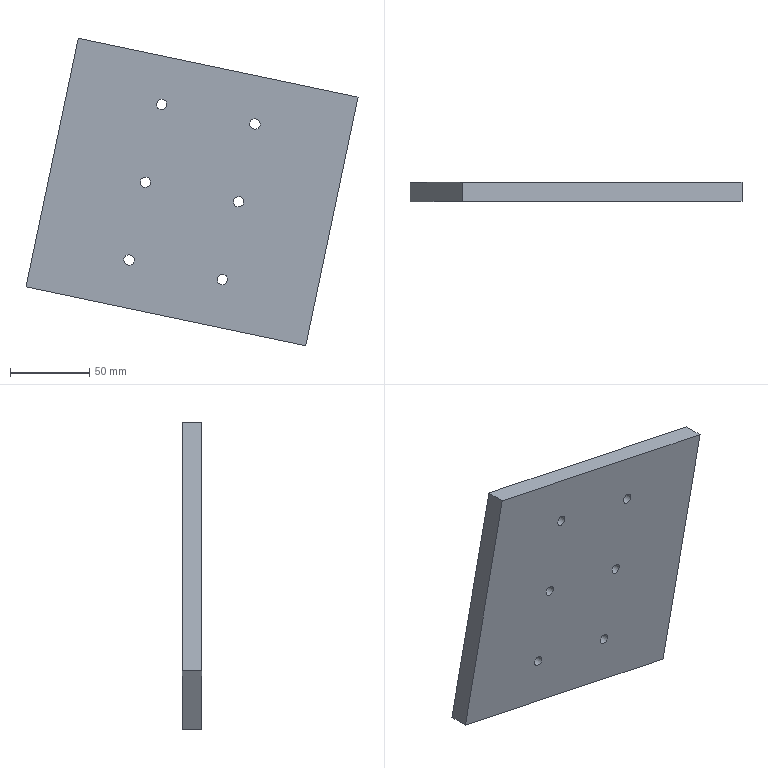Part | STEP file | SOLID | 1 solid | 24 faces | box 209.056 x 12 x 193.596 mm | volume 339030 mm3 | plane 12 | cylinder 12 | commonest cylinder face diameters 6.5 x6 13 x6
STEP:
#1=CARTESIAN_POINT('',(0.,0.,0.));
#2=DIRECTION('',(0.,0.,1.));
#3=DIRECTION('',(1.,0.,0.));
#4=AXIS2_PLACEMENT_3D('',#1,#2,#3);
#5=CARTESIAN_POINT('',(-554.568,-704.15,575.987));
#6=VERTEX_POINT('',#5);
#7=CARTESIAN_POINT('',(-560.929,-704.15,577.323));
#8=DIRECTION('',(0.,1.,0.));
#9=DIRECTION('',(0.9786,0.,-0.2056));
#10=AXIS2_PLACEMENT_3D('',#7,#8,#9);
#11=CIRCLE('',#10,6.5);
#12=CARTESIAN_POINT('',(-560.929,-704.15,577.323));
#13=DIRECTION('',(0.,1.,0.));
#14=DIRECTION('',(0.9786,0.,-0.2056));
#15=AXIS2_PLACEMENT_3D('',#12,#13,#14);
#16=PLANE('',#15);
#17=CARTESIAN_POINT('',(0.,0.));
#18=DIRECTION('',(1.,0.));
#19=AXIS2_PLACEMENT_2D('',#17,#18);
#20=CIRCLE('',#19,6.5);
#21=(GEOMETRIC_REPRESENTATION_CONTEXT(2)PARAMETRIC_REPRESENTATION_CONTEXT()REPRESENTATION_CONTEXT('',''));
#22=DEFINITIONAL_REPRESENTATION('',(#20),#21);
#23=PCURVE('',#16,#22);
#24=CARTESIAN_POINT('',(-560.929,-700.65,577.323));
#25=DIRECTION('',(0.,1.,0.));
#26=DIRECTION('',(0.9786,0.,-0.2056));
#27=AXIS2_PLACEMENT_3D('',#24,#25,#26);
#28=CYLINDRICAL_SURFACE('',#27,6.5);
#29=CARTESIAN_POINT('',(0.,-3.5));
#30=DIRECTION('',(1.,0.));
#31=VECTOR('',#30,1.);
#32=LINE('',#29,#31);
#33=(GEOMETRIC_REPRESENTATION_CONTEXT(2)PARAMETRIC_REPRESENTATION_CONTEXT()REPRESENTATION_CONTEXT('',''));
#34=DEFINITIONAL_REPRESENTATION('',(#32),#33);
#35=PCURVE('',#28,#34);
#36=SURFACE_CURVE('',#11,(#23,#35),.PCURVE_S1.);
#37=EDGE_CURVE('',#6,#6,#36,.T.);
#38=ORIENTED_EDGE('',*,*,#37,.T.);
#39=EDGE_LOOP('',(#38));
#40=FACE_BOUND('',#39,.T.);
#41=CARTESIAN_POINT('',(-564.11,-704.15,577.992));
#42=VERTEX_POINT('',#41);
#43=CARTESIAN_POINT('',(-560.929,-704.15,577.323));
#44=DIRECTION('',(0.,1.,0.));
#45=DIRECTION('',(0.9786,0.,-0.2056));
#46=AXIS2_PLACEMENT_3D('',#43,#44,#45);
#47=CIRCLE('',#46,3.25);
#48=CARTESIAN_POINT('',(0.,0.));
#49=DIRECTION('',(1.,0.));
#50=AXIS2_PLACEMENT_2D('',#48,#49);
#51=CIRCLE('',#50,3.25);
#52=(GEOMETRIC_REPRESENTATION_CONTEXT(2)PARAMETRIC_REPRESENTATION_CONTEXT()REPRESENTATION_CONTEXT('',''));
#53=DEFINITIONAL_REPRESENTATION('',(#51),#52);
#54=PCURVE('',#16,#53);
#55=CARTESIAN_POINT('',(-560.929,-982.33,577.323));
#56=DIRECTION('',(0.,1.,0.));
#57=DIRECTION('',(0.9786,0.,-0.2056));
#58=AXIS2_PLACEMENT_3D('',#55,#56,#57);
#59=CYLINDRICAL_SURFACE('',#58,3.25);
#60=CARTESIAN_POINT('',(0.,278.18));
#61=DIRECTION('',(1.,0.));
#62=VECTOR('',#61,1.);
#63=LINE('',#60,#62);
#64=(GEOMETRIC_REPRESENTATION_CONTEXT(2)PARAMETRIC_REPRESENTATION_CONTEXT()REPRESENTATION_CONTEXT('',''));
#65=DEFINITIONAL_REPRESENTATION('',(#63),#64);
#66=PCURVE('',#59,#65);
#67=SURFACE_CURVE('',#47,(#54,#66),.PCURVE_S1.);
#68=EDGE_CURVE('',#42,#42,#67,.T.);
#69=ORIENTED_EDGE('',*,*,#68,.F.);
#70=EDGE_LOOP('',(#69));
#71=FACE_BOUND('',#70,.T.);
#72=ADVANCED_FACE('',(#40,#71),#16,.T.);
#73=CARTESIAN_POINT('',(-554.568,-697.15,575.987));
#74=VERTEX_POINT('',#73);
#75=CARTESIAN_POINT('',(-560.929,-697.15,577.323));
#76=DIRECTION('',(0.,-1.,0.));
#77=DIRECTION('',(0.9786,0.,-0.2056));
#78=AXIS2_PLACEMENT_3D('',#75,#76,#77);
#79=CIRCLE('',#78,6.5);
#80=CARTESIAN_POINT('',(6.283,3.5));
#81=DIRECTION('',(-1.,0.));
#82=VECTOR('',#81,1.);
#83=LINE('',#80,#82);
#84=(GEOMETRIC_REPRESENTATION_CONTEXT(2)PARAMETRIC_REPRESENTATION_CONTEXT()REPRESENTATION_CONTEXT('',''));
#85=DEFINITIONAL_REPRESENTATION('',(#83),#84);
#86=PCURVE('',#28,#85);
#87=CARTESIAN_POINT('',(-672.195,-697.15,631.359));
#88=DIRECTION('',(0.,-1.,0.));
#89=DIRECTION('',(0.,0.,-1.));
#90=AXIS2_PLACEMENT_3D('',#87,#88,#89);
#91=PLANE('',#90);
#92=CARTESIAN_POINT('',(54.036,111.266));
#93=DIRECTION('',(0.2056,0.9786));
#94=AXIS2_PLACEMENT_2D('',#92,#93);
#95=CIRCLE('',#94,6.5);
#96=(GEOMETRIC_REPRESENTATION_CONTEXT(2)PARAMETRIC_REPRESENTATION_CONTEXT()REPRESENTATION_CONTEXT('',''));
#97=DEFINITIONAL_REPRESENTATION('',(#95),#96);
#98=PCURVE('',#91,#97);
#99=SURFACE_CURVE('',#79,(#86,#98),.PCURVE_S1.);
#100=EDGE_CURVE('',#74,#74,#99,.T.);
#101=ORIENTED_EDGE('',*,*,#100,.T.);
#102=CARTESIAN_POINT('',(-554.568,-704.15,575.987));
#103=CARTESIAN_POINT('',(-554.568,-697.15,575.987));
#104=B_SPLINE_CURVE_WITH_KNOTS('',1,(#102,#103),.UNSPECIFIED.,.F.,.F.,(2,2),(-3.5,3.5),.PIECEWISE_BEZIER_KNOTS.);
#105=CARTESIAN_POINT('',(0.,0.));
#106=DIRECTION('',(0.,1.));
#107=VECTOR('',#106,1.);
#108=LINE('',#105,#107);
#109=(GEOMETRIC_REPRESENTATION_CONTEXT(2)PARAMETRIC_REPRESENTATION_CONTEXT()REPRESENTATION_CONTEXT('',''));
#110=DEFINITIONAL_REPRESENTATION('',(#108),#109);
#111=PCURVE('',#28,#110);
#112=CARTESIAN_POINT('',(6.283,0.));
#113=DIRECTION('',(0.,1.));
#114=VECTOR('',#113,1.);
#115=LINE('',#112,#114);
#116=(GEOMETRIC_REPRESENTATION_CONTEXT(2)PARAMETRIC_REPRESENTATION_CONTEXT()REPRESENTATION_CONTEXT('',''));
#117=DEFINITIONAL_REPRESENTATION('',(#115),#116);
#118=PCURVE('',#28,#117);
#119=SEAM_CURVE('',#104,(#111,#118),.PCURVE_S1.);
#120=EDGE_CURVE('',#6,#74,#119,.T.);
#121=ORIENTED_EDGE('',*,*,#120,.F.);
#122=ORIENTED_EDGE('',*,*,#37,.T.);
#123=ORIENTED_EDGE('',*,*,#120,.T.);
#124=EDGE_LOOP('',(#101,#121,#122,#123));
#125=FACE_BOUND('',#124,.F.);
#126=ADVANCED_FACE('',(#125),#28,.F.);
#127=CARTESIAN_POINT('',(-564.11,-709.15,577.992));
#128=VERTEX_POINT('',#127);
#129=CARTESIAN_POINT('',(-560.929,-709.15,577.323));
#130=DIRECTION('',(0.,1.,0.));
#131=DIRECTION('',(0.9786,0.,-0.2056));
#132=AXIS2_PLACEMENT_3D('',#129,#130,#131);
#133=CIRCLE('',#132,3.25);
#134=CARTESIAN_POINT('',(0.,273.18));
#135=DIRECTION('',(1.,0.));
#136=VECTOR('',#135,1.);
#137=LINE('',#134,#136);
#138=(GEOMETRIC_REPRESENTATION_CONTEXT(2)PARAMETRIC_REPRESENTATION_CONTEXT()REPRESENTATION_CONTEXT('',''));
#139=DEFINITIONAL_REPRESENTATION('',(#137),#138);
#140=PCURVE('',#59,#139);
#141=CARTESIAN_POINT('',(-554.191,-709.15,463.505));
#142=DIRECTION('',(0.,1.,0.));
#143=DIRECTION('',(0.,0.,1.));
#144=AXIS2_PLACEMENT_3D('',#141,#142,#143);
#145=PLANE('',#144);
#146=CARTESIAN_POINT('',(113.818,-6.738));
#147=DIRECTION('',(-0.2056,0.9786));
#148=AXIS2_PLACEMENT_2D('',#146,#147);
#149=CIRCLE('',#148,3.25);
#150=(GEOMETRIC_REPRESENTATION_CONTEXT(2)PARAMETRIC_REPRESENTATION_CONTEXT()REPRESENTATION_CONTEXT('',''));
#151=DEFINITIONAL_REPRESENTATION('',(#149),#150);
#152=PCURVE('',#145,#151);
#153=SURFACE_CURVE('',#133,(#140,#152),.PCURVE_S1.);
#154=EDGE_CURVE('',#128,#128,#153,.T.);
#155=ORIENTED_EDGE('',*,*,#154,.T.);
#156=CARTESIAN_POINT('',(-564.11,-709.15,577.992));
#157=CARTESIAN_POINT('',(-564.11,-704.15,577.992));
#158=B_SPLINE_CURVE_WITH_KNOTS('',1,(#156,#157),.UNSPECIFIED.,.F.,.F.,(2,2),(273.18,278.18),.PIECEWISE_BEZIER_KNOTS.);
#159=CARTESIAN_POINT('',(9.425,0.));
#160=DIRECTION('',(0.,1.));
#161=VECTOR('',#160,1.);
#162=LINE('',#159,#161);
#163=(GEOMETRIC_REPRESENTATION_CONTEXT(2)PARAMETRIC_REPRESENTATION_CONTEXT()REPRESENTATION_CONTEXT('',''));
#164=DEFINITIONAL_REPRESENTATION('',(#162),#163);
#165=PCURVE('',#59,#164);
#166=CARTESIAN_POINT('',(3.142,0.));
#167=DIRECTION('',(0.,1.));
#168=VECTOR('',#167,1.);
#169=LINE('',#166,#168);
#170=(GEOMETRIC_REPRESENTATION_CONTEXT(2)PARAMETRIC_REPRESENTATION_CONTEXT()REPRESENTATION_CONTEXT('',''));
#171=DEFINITIONAL_REPRESENTATION('',(#169),#170);
#172=PCURVE('',#59,#171);
#173=SEAM_CURVE('',#158,(#165,#172),.PCURVE_S1.);
#174=EDGE_CURVE('',#128,#42,#173,.T.);
#175=ORIENTED_EDGE('',*,*,#174,.T.);
#176=ORIENTED_EDGE('',*,*,#68,.F.);
#177=ORIENTED_EDGE('',*,*,#174,.F.);
#178=EDGE_LOOP('',(#155,#175,#176,#177));
#179=FACE_BOUND('',#178,.F.);
#180=ADVANCED_FACE('',(#179),#59,.F.);
#181=CARTESIAN_POINT('',(-564.85,-704.15,527.055));
#182=VERTEX_POINT('',#181);
#183=CARTESIAN_POINT('',(-571.211,-704.15,528.392));
#184=DIRECTION('',(0.,1.,0.));
#185=DIRECTION('',(0.9786,0.,-0.2056));
#186=AXIS2_PLACEMENT_3D('',#183,#184,#185);
#187=CIRCLE('',#186,6.5);
#188=CARTESIAN_POINT('',(-571.211,-704.15,528.392));
#189=DIRECTION('',(0.,1.,0.));
#190=DIRECTION('',(0.9786,0.,-0.2056));
#191=AXIS2_PLACEMENT_3D('',#188,#189,#190);
#192=PLANE('',#191);
#193=CARTESIAN_POINT('',(0.,0.));
#194=DIRECTION('',(1.,0.));
#195=AXIS2_PLACEMENT_2D('',#193,#194);
#196=CIRCLE('',#195,6.5);
#197=(GEOMETRIC_REPRESENTATION_CONTEXT(2)PARAMETRIC_REPRESENTATION_CONTEXT()REPRESENTATION_CONTEXT('',''));
#198=DEFINITIONAL_REPRESENTATION('',(#196),#197);
#199=PCURVE('',#192,#198);
#200=CARTESIAN_POINT('',(-571.211,-700.65,528.392));
#201=DIRECTION('',(0.,1.,0.));
#202=DIRECTION('',(0.9786,0.,-0.2056));
#203=AXIS2_PLACEMENT_3D('',#200,#201,#202);
#204=CYLINDRICAL_SURFACE('',#203,6.5);
#205=CARTESIAN_POINT('',(0.,-3.5));
#206=DIRECTION('',(1.,0.));
#207=VECTOR('',#206,1.);
#208=LINE('',#205,#207);
#209=(GEOMETRIC_REPRESENTATION_CONTEXT(2)PARAMETRIC_REPRESENTATION_CONTEXT()REPRESENTATION_CONTEXT('',''));
#210=DEFINITIONAL_REPRESENTATION('',(#208),#209);
#211=PCURVE('',#204,#210);
#212=SURFACE_CURVE('',#187,(#199,#211),.PCURVE_S1.);
#213=EDGE_CURVE('',#182,#182,#212,.T.);
#214=ORIENTED_EDGE('',*,*,#213,.T.);
#215=EDGE_LOOP('',(#214));
#216=FACE_BOUND('',#215,.T.);
#217=CARTESIAN_POINT('',(-574.392,-704.15,529.06));
#218=VERTEX_POINT('',#217);
#219=CARTESIAN_POINT('',(-571.211,-704.15,528.392));
#220=DIRECTION('',(0.,1.,0.));
#221=DIRECTION('',(0.9786,0.,-0.2056));
#222=AXIS2_PLACEMENT_3D('',#219,#220,#221);
#223=CIRCLE('',#222,3.25);
#224=CARTESIAN_POINT('',(0.,0.));
#225=DIRECTION('',(1.,0.));
#226=AXIS2_PLACEMENT_2D('',#224,#225);
#227=CIRCLE('',#226,3.25);
#228=(GEOMETRIC_REPRESENTATION_CONTEXT(2)PARAMETRIC_REPRESENTATION_CONTEXT()REPRESENTATION_CONTEXT('',''));
#229=DEFINITIONAL_REPRESENTATION('',(#227),#228);
#230=PCURVE('',#192,#229);
#231=CARTESIAN_POINT('',(-571.211,-982.33,528.392));
#232=DIRECTION('',(0.,1.,0.));
#233=DIRECTION('',(0.9786,0.,-0.2056));
#234=AXIS2_PLACEMENT_3D('',#231,#232,#233);
#235=CYLINDRICAL_SURFACE('',#234,3.25);
#236=CARTESIAN_POINT('',(0.,278.18));
#237=DIRECTION('',(1.,0.));
#238=VECTOR('',#237,1.);
#239=LINE('',#236,#238);
#240=(GEOMETRIC_REPRESENTATION_CONTEXT(2)PARAMETRIC_REPRESENTATION_CONTEXT()REPRESENTATION_CONTEXT('',''));
#241=DEFINITIONAL_REPRESENTATION('',(#239),#240);
#242=PCURVE('',#235,#241);
#243=SURFACE_CURVE('',#223,(#230,#242),.PCURVE_S1.);
#244=EDGE_CURVE('',#218,#218,#243,.T.);
#245=ORIENTED_EDGE('',*,*,#244,.F.);
#246=EDGE_LOOP('',(#245));
#247=FACE_BOUND('',#246,.T.);
#248=ADVANCED_FACE('',(#216,#247),#192,.T.);
#249=CARTESIAN_POINT('',(-564.85,-697.15,527.055));
#250=VERTEX_POINT('',#249);
#251=CARTESIAN_POINT('',(-571.211,-697.15,528.392));
#252=DIRECTION('',(0.,-1.,0.));
#253=DIRECTION('',(0.9786,0.,-0.2056));
#254=AXIS2_PLACEMENT_3D('',#251,#252,#253);
#255=CIRCLE('',#254,6.5);
#256=CARTESIAN_POINT('',(6.283,3.5));
#257=DIRECTION('',(-1.,0.));
#258=VECTOR('',#257,1.);
#259=LINE('',#256,#258);
#260=(GEOMETRIC_REPRESENTATION_CONTEXT(2)PARAMETRIC_REPRESENTATION_CONTEXT()REPRESENTATION_CONTEXT('',''));
#261=DEFINITIONAL_REPRESENTATION('',(#259),#260);
#262=PCURVE('',#204,#261);
#263=CARTESIAN_POINT('',(102.967,100.984));
#264=DIRECTION('',(0.2056,0.9786));
#265=AXIS2_PLACEMENT_2D('',#263,#264);
#266=CIRCLE('',#265,6.5);
#267=(GEOMETRIC_REPRESENTATION_CONTEXT(2)PARAMETRIC_REPRESENTATION_CONTEXT()REPRESENTATION_CONTEXT('',''));
#268=DEFINITIONAL_REPRESENTATION('',(#266),#267);
#269=PCURVE('',#91,#268);
#270=SURFACE_CURVE('',#255,(#262,#269),.PCURVE_S1.);
#271=EDGE_CURVE('',#250,#250,#270,.T.);
#272=ORIENTED_EDGE('',*,*,#271,.T.);
#273=CARTESIAN_POINT('',(-564.85,-704.15,527.055));
#274=CARTESIAN_POINT('',(-564.85,-697.15,527.055));
#275=B_SPLINE_CURVE_WITH_KNOTS('',1,(#273,#274),.UNSPECIFIED.,.F.,.F.,(2,2),(-3.5,3.5),.PIECEWISE_BEZIER_KNOTS.);
#276=CARTESIAN_POINT('',(0.,0.));
#277=DIRECTION('',(0.,1.));
#278=VECTOR('',#277,1.);
#279=LINE('',#276,#278);
#280=(GEOMETRIC_REPRESENTATION_CONTEXT(2)PARAMETRIC_REPRESENTATION_CONTEXT()REPRESENTATION_CONTEXT('',''));
#281=DEFINITIONAL_REPRESENTATION('',(#279),#280);
#282=PCURVE('',#204,#281);
#283=CARTESIAN_POINT('',(6.283,0.));
#284=DIRECTION('',(0.,1.));
#285=VECTOR('',#284,1.);
#286=LINE('',#283,#285);
#287=(GEOMETRIC_REPRESENTATION_CONTEXT(2)PARAMETRIC_REPRESENTATION_CONTEXT()REPRESENTATION_CONTEXT('',''));
#288=DEFINITIONAL_REPRESENTATION('',(#286),#287);
#289=PCURVE('',#204,#288);
#290=SEAM_CURVE('',#275,(#282,#289),.PCURVE_S1.);
#291=EDGE_CURVE('',#182,#250,#290,.T.);
#292=ORIENTED_EDGE('',*,*,#291,.F.);
#293=ORIENTED_EDGE('',*,*,#213,.T.);
#294=ORIENTED_EDGE('',*,*,#291,.T.);
#295=EDGE_LOOP('',(#272,#292,#293,#294));
#296=FACE_BOUND('',#295,.F.);
#297=ADVANCED_FACE('',(#296),#204,.F.);
#298=CARTESIAN_POINT('',(-574.392,-709.15,529.06));
#299=VERTEX_POINT('',#298);
#300=CARTESIAN_POINT('',(-571.211,-709.15,528.392));
#301=DIRECTION('',(0.,1.,0.));
#302=DIRECTION('',(0.9786,0.,-0.2056));
#303=AXIS2_PLACEMENT_3D('',#300,#301,#302);
#304=CIRCLE('',#303,3.25);
#305=CARTESIAN_POINT('',(0.,273.18));
#306=DIRECTION('',(1.,0.));
#307=VECTOR('',#306,1.);
#308=LINE('',#305,#307);
#309=(GEOMETRIC_REPRESENTATION_CONTEXT(2)PARAMETRIC_REPRESENTATION_CONTEXT()REPRESENTATION_CONTEXT('',''));
#310=DEFINITIONAL_REPRESENTATION('',(#308),#309);
#311=PCURVE('',#235,#310);
#312=CARTESIAN_POINT('',(64.887,-17.02));
#313=DIRECTION('',(-0.2056,0.9786));
#314=AXIS2_PLACEMENT_2D('',#312,#313);
#315=CIRCLE('',#314,3.25);
#316=(GEOMETRIC_REPRESENTATION_CONTEXT(2)PARAMETRIC_REPRESENTATION_CONTEXT()REPRESENTATION_CONTEXT('',''));
#317=DEFINITIONAL_REPRESENTATION('',(#315),#316);
#318=PCURVE('',#145,#317);
#319=SURFACE_CURVE('',#304,(#311,#318),.PCURVE_S1.);
#320=EDGE_CURVE('',#299,#299,#319,.T.);
#321=ORIENTED_EDGE('',*,*,#320,.T.);
#322=CARTESIAN_POINT('',(-574.392,-709.15,529.06));
#323=CARTESIAN_POINT('',(-574.392,-704.15,529.06));
#324=B_SPLINE_CURVE_WITH_KNOTS('',1,(#322,#323),.UNSPECIFIED.,.F.,.F.,(2,2),(273.18,278.18),.PIECEWISE_BEZIER_KNOTS.);
#325=CARTESIAN_POINT('',(9.425,0.));
#326=DIRECTION('',(0.,1.));
#327=VECTOR('',#326,1.);
#328=LINE('',#325,#327);
#329=(GEOMETRIC_REPRESENTATION_CONTEXT(2)PARAMETRIC_REPRESENTATION_CONTEXT()REPRESENTATION_CONTEXT('',''));
#330=DEFINITIONAL_REPRESENTATION('',(#328),#329);
#331=PCURVE('',#235,#330);
#332=CARTESIAN_POINT('',(3.142,0.));
#333=DIRECTION('',(0.,1.));
#334=VECTOR('',#333,1.);
#335=LINE('',#332,#334);
#336=(GEOMETRIC_REPRESENTATION_CONTEXT(2)PARAMETRIC_REPRESENTATION_CONTEXT()REPRESENTATION_CONTEXT('',''));
#337=DEFINITIONAL_REPRESENTATION('',(#335),#336);
#338=PCURVE('',#235,#337);
#339=SEAM_CURVE('',#324,(#331,#338),.PCURVE_S1.);
#340=EDGE_CURVE('',#299,#218,#339,.T.);
#341=ORIENTED_EDGE('',*,*,#340,.T.);
#342=ORIENTED_EDGE('',*,*,#244,.F.);
#343=ORIENTED_EDGE('',*,*,#340,.F.);
#344=EDGE_LOOP('',(#321,#341,#342,#343));
#345=FACE_BOUND('',#344,.F.);
#346=ADVANCED_FACE('',(#345),#235,.F.);
#347=CARTESIAN_POINT('',(-575.132,-704.15,478.124));
#348=VERTEX_POINT('',#347);
#349=CARTESIAN_POINT('',(-581.494,-704.15,479.46));
#350=DIRECTION('',(0.,1.,0.));
#351=DIRECTION('',(0.9786,0.,-0.2056));
#352=AXIS2_PLACEMENT_3D('',#349,#350,#351);
#353=CIRCLE('',#352,6.5);
#354=CARTESIAN_POINT('',(-581.494,-704.15,479.46));
#355=DIRECTION('',(0.,1.,0.));
#356=DIRECTION('',(0.9786,0.,-0.2056));
#357=AXIS2_PLACEMENT_3D('',#354,#355,#356);
#358=PLANE('',#357);
#359=CARTESIAN_POINT('',(0.,0.));
#360=DIRECTION('',(1.,0.));
#361=AXIS2_PLACEMENT_2D('',#359,#360);
#362=CIRCLE('',#361,6.5);
#363=(GEOMETRIC_REPRESENTATION_CONTEXT(2)PARAMETRIC_REPRESENTATION_CONTEXT()REPRESENTATION_CONTEXT('',''));
#364=DEFINITIONAL_REPRESENTATION('',(#362),#363);
#365=PCURVE('',#358,#364);
#366=CARTESIAN_POINT('',(-581.494,-700.65,479.46));
#367=DIRECTION('',(0.,1.,0.));
#368=DIRECTION('',(0.9786,0.,-0.2056));
#369=AXIS2_PLACEMENT_3D('',#366,#367,#368);
#370=CYLINDRICAL_SURFACE('',#369,6.5);
#371=CARTESIAN_POINT('',(0.,-3.5));
#372=DIRECTION('',(1.,0.));
#373=VECTOR('',#372,1.);
#374=LINE('',#371,#373);
#375=(GEOMETRIC_REPRESENTATION_CONTEXT(2)PARAMETRIC_REPRESENTATION_CONTEXT()REPRESENTATION_CONTEXT('',''));
#376=DEFINITIONAL_REPRESENTATION('',(#374),#375);
#377=PCURVE('',#370,#376);
#378=SURFACE_CURVE('',#353,(#365,#377),.PCURVE_S1.);
#379=EDGE_CURVE('',#348,#348,#378,.T.);
#380=ORIENTED_EDGE('',*,*,#379,.T.);
#381=EDGE_LOOP('',(#380));
#382=FACE_BOUND('',#381,.T.);
#383=CARTESIAN_POINT('',(-584.674,-704.15,480.129));
#384=VERTEX_POINT('',#383);
#385=CARTESIAN_POINT('',(-581.494,-704.15,479.46));
#386=DIRECTION('',(0.,1.,0.));
#387=DIRECTION('',(0.9786,0.,-0.2056));
#388=AXIS2_PLACEMENT_3D('',#385,#386,#387);
#389=CIRCLE('',#388,3.25);
#390=CARTESIAN_POINT('',(0.,0.));
#391=DIRECTION('',(1.,0.));
#392=AXIS2_PLACEMENT_2D('',#390,#391);
#393=CIRCLE('',#392,3.25);
#394=(GEOMETRIC_REPRESENTATION_CONTEXT(2)PARAMETRIC_REPRESENTATION_CONTEXT()REPRESENTATION_CONTEXT('',''));
#395=DEFINITIONAL_REPRESENTATION('',(#393),#394);
#396=PCURVE('',#358,#395);
#397=CARTESIAN_POINT('',(-581.494,-982.33,479.46));
#398=DIRECTION('',(0.,1.,0.));
#399=DIRECTION('',(0.9786,0.,-0.2056));
#400=AXIS2_PLACEMENT_3D('',#397,#398,#399);
#401=CYLINDRICAL_SURFACE('',#400,3.25);
#402=CARTESIAN_POINT('',(0.,278.18));
#403=DIRECTION('',(1.,0.));
#404=VECTOR('',#403,1.);
#405=LINE('',#402,#404);
#406=(GEOMETRIC_REPRESENTATION_CONTEXT(2)PARAMETRIC_REPRESENTATION_CONTEXT()REPRESENTATION_CONTEXT('',''));
#407=DEFINITIONAL_REPRESENTATION('',(#405),#406);
#408=PCURVE('',#401,#407);
#409=SURFACE_CURVE('',#389,(#396,#408),.PCURVE_S1.);
#410=EDGE_CURVE('',#384,#384,#409,.T.);
#411=ORIENTED_EDGE('',*,*,#410,.F.);
#412=EDGE_LOOP('',(#411));
#413=FACE_BOUND('',#412,.T.);
#414=ADVANCED_FACE('',(#382,#413),#358,.T.);
#415=CARTESIAN_POINT('',(-575.132,-697.15,478.124));
#416=VERTEX_POINT('',#415);
#417=CARTESIAN_POINT('',(-581.494,-697.15,479.46));
#418=DIRECTION('',(0.,-1.,0.));
#419=DIRECTION('',(0.9786,0.,-0.2056));
#420=AXIS2_PLACEMENT_3D('',#417,#418,#419);
#421=CIRCLE('',#420,6.5);
#422=CARTESIAN_POINT('',(6.283,3.5));
#423=DIRECTION('',(-1.,0.));
#424=VECTOR('',#423,1.);
#425=LINE('',#422,#424);
#426=(GEOMETRIC_REPRESENTATION_CONTEXT(2)PARAMETRIC_REPRESENTATION_CONTEXT()REPRESENTATION_CONTEXT('',''));
#427=DEFINITIONAL_REPRESENTATION('',(#425),#426);
#428=PCURVE('',#370,#427);
#429=CARTESIAN_POINT('',(151.899,90.702));
#430=DIRECTION('',(0.2056,0.9786));
#431=AXIS2_PLACEMENT_2D('',#429,#430);
#432=CIRCLE('',#431,6.5);
#433=(GEOMETRIC_REPRESENTATION_CONTEXT(2)PARAMETRIC_REPRESENTATION_CONTEXT()REPRESENTATION_CONTEXT('',''));
#434=DEFINITIONAL_REPRESENTATION('',(#432),#433);
#435=PCURVE('',#91,#434);
#436=SURFACE_CURVE('',#421,(#428,#435),.PCURVE_S1.);
#437=EDGE_CURVE('',#416,#416,#436,.T.);
#438=ORIENTED_EDGE('',*,*,#437,.T.);
#439=CARTESIAN_POINT('',(-575.132,-704.15,478.124));
#440=CARTESIAN_POINT('',(-575.132,-697.15,478.124));
#441=B_SPLINE_CURVE_WITH_KNOTS('',1,(#439,#440),.UNSPECIFIED.,.F.,.F.,(2,2),(-3.5,3.5),.PIECEWISE_BEZIER_KNOTS.);
#442=CARTESIAN_POINT('',(0.,0.));
#443=DIRECTION('',(0.,1.));
#444=VECTOR('',#443,1.);
#445=LINE('',#442,#444);
#446=(GEOMETRIC_REPRESENTATION_CONTEXT(2)PARAMETRIC_REPRESENTATION_CONTEXT()REPRESENTATION_CONTEXT('',''));
#447=DEFINITIONAL_REPRESENTATION('',(#445),#446);
#448=PCURVE('',#370,#447);
#449=CARTESIAN_POINT('',(6.283,0.));
#450=DIRECTION('',(0.,1.));
#451=VECTOR('',#450,1.);
#452=LINE('',#449,#451);
#453=(GEOMETRIC_REPRESENTATION_CONTEXT(2)PARAMETRIC_REPRESENTATION_CONTEXT()REPRESENTATION_CONTEXT('',''));
#454=DEFINITIONAL_REPRESENTATION('',(#452),#453);
#455=PCURVE('',#370,#454);
#456=SEAM_CURVE('',#441,(#448,#455),.PCURVE_S1.);
#457=EDGE_CURVE('',#348,#416,#456,.T.);
#458=ORIENTED_EDGE('',*,*,#457,.F.);
#459=ORIENTED_EDGE('',*,*,#379,.T.);
#460=ORIENTED_EDGE('',*,*,#457,.T.);
#461=EDGE_LOOP('',(#438,#458,#459,#460));
#462=FACE_BOUND('',#461,.F.);
#463=ADVANCED_FACE('',(#462),#370,.F.);
#464=CARTESIAN_POINT('',(-584.674,-709.15,480.129));
#465=VERTEX_POINT('',#464);
#466=CARTESIAN_POINT('',(-581.494,-709.15,479.46));
#467=DIRECTION('',(0.,1.,0.));
#468=DIRECTION('',(0.9786,0.,-0.2056));
#469=AXIS2_PLACEMENT_3D('',#466,#467,#468);
#470=CIRCLE('',#469,3.25);
#471=CARTESIAN_POINT('',(0.,273.18));
#472=DIRECTION('',(1.,0.));
#473=VECTOR('',#472,1.);
#474=LINE('',#471,#473);
#475=(GEOMETRIC_REPRESENTATION_CONTEXT(2)PARAMETRIC_REPRESENTATION_CONTEXT()REPRESENTATION_CONTEXT('',''));
#476=DEFINITIONAL_REPRESENTATION('',(#474),#475);
#477=PCURVE('',#401,#476);
#478=CARTESIAN_POINT('',(15.956,-27.302));
#479=DIRECTION('',(-0.2056,0.9786));
#480=AXIS2_PLACEMENT_2D('',#478,#479);
#481=CIRCLE('',#480,3.25);
#482=(GEOMETRIC_REPRESENTATION_CONTEXT(2)PARAMETRIC_REPRESENTATION_CONTEXT()REPRESENTATION_CONTEXT('',''));
#483=DEFINITIONAL_REPRESENTATION('',(#481),#482);
#484=PCURVE('',#145,#483);
#485=SURFACE_CURVE('',#470,(#477,#484),.PCURVE_S1.);
#486=EDGE_CURVE('',#465,#465,#485,.T.);
#487=ORIENTED_EDGE('',*,*,#486,.T.);
#488=CARTESIAN_POINT('',(-584.674,-709.15,480.129));
#489=CARTESIAN_POINT('',(-584.674,-704.15,480.129));
#490=B_SPLINE_CURVE_WITH_KNOTS('',1,(#488,#489),.UNSPECIFIED.,.F.,.F.,(2,2),(273.18,278.18),.PIECEWISE_BEZIER_KNOTS.);
#491=CARTESIAN_POINT('',(9.425,0.));
#492=DIRECTION('',(0.,1.));
#493=VECTOR('',#492,1.);
#494=LINE('',#491,#493);
#495=(GEOMETRIC_REPRESENTATION_CONTEXT(2)PARAMETRIC_REPRESENTATION_CONTEXT()REPRESENTATION_CONTEXT('',''));
#496=DEFINITIONAL_REPRESENTATION('',(#494),#495);
#497=PCURVE('',#401,#496);
#498=CARTESIAN_POINT('',(3.142,0.));
#499=DIRECTION('',(0.,1.));
#500=VECTOR('',#499,1.);
#501=LINE('',#498,#500);
#502=(GEOMETRIC_REPRESENTATION_CONTEXT(2)PARAMETRIC_REPRESENTATION_CONTEXT()REPRESENTATION_CONTEXT('',''));
#503=DEFINITIONAL_REPRESENTATION('',(#501),#502);
#504=PCURVE('',#401,#503);
#505=SEAM_CURVE('',#490,(#497,#504),.PCURVE_S1.);
#506=EDGE_CURVE('',#465,#384,#505,.T.);
#507=ORIENTED_EDGE('',*,*,#506,.T.);
#508=ORIENTED_EDGE('',*,*,#410,.F.);
#509=ORIENTED_EDGE('',*,*,#506,.F.);
#510=EDGE_LOOP('',(#487,#507,#508,#509));
#511=FACE_BOUND('',#510,.F.);
#512=ADVANCED_FACE('',(#511),#401,.F.);
#513=CARTESIAN_POINT('',(-633.85,-704.15,490.462));
#514=VERTEX_POINT('',#513);
#515=CARTESIAN_POINT('',(-640.211,-704.15,491.799));
#516=DIRECTION('',(0.,1.,0.));
#517=DIRECTION('',(0.9786,0.,-0.2056));
#518=AXIS2_PLACEMENT_3D('',#515,#516,#517);
#519=CIRCLE('',#518,6.5);
#520=CARTESIAN_POINT('',(-640.211,-704.15,491.799));
#521=DIRECTION('',(0.,1.,0.));
#522=DIRECTION('',(0.9786,0.,-0.2056));
#523=AXIS2_PLACEMENT_3D('',#520,#521,#522);
#524=PLANE('',#523);
#525=CARTESIAN_POINT('',(0.,0.));
#526=DIRECTION('',(1.,0.));
#527=AXIS2_PLACEMENT_2D('',#525,#526);
#528=CIRCLE('',#527,6.5);
#529=(GEOMETRIC_REPRESENTATION_CONTEXT(2)PARAMETRIC_REPRESENTATION_CONTEXT()REPRESENTATION_CONTEXT('',''));
#530=DEFINITIONAL_REPRESENTATION('',(#528),#529);
#531=PCURVE('',#524,#530);
#532=CARTESIAN_POINT('',(-640.211,-700.65,491.799));
#533=DIRECTION('',(0.,1.,0.));
#534=DIRECTION('',(0.9786,0.,-0.2056));
#535=AXIS2_PLACEMENT_3D('',#532,#533,#534);
#536=CYLINDRICAL_SURFACE('',#535,6.5);
#537=CARTESIAN_POINT('',(0.,-3.5));
#538=DIRECTION('',(1.,0.));
#539=VECTOR('',#538,1.);
#540=LINE('',#537,#539);
#541=(GEOMETRIC_REPRESENTATION_CONTEXT(2)PARAMETRIC_REPRESENTATION_CONTEXT()REPRESENTATION_CONTEXT('',''));
#542=DEFINITIONAL_REPRESENTATION('',(#540),#541);
#543=PCURVE('',#536,#542);
#544=SURFACE_CURVE('',#519,(#531,#543),.PCURVE_S1.);
#545=EDGE_CURVE('',#514,#514,#544,.T.);
#546=ORIENTED_EDGE('',*,*,#545,.T.);
#547=EDGE_LOOP('',(#546));
#548=FACE_BOUND('',#547,.T.);
#549=CARTESIAN_POINT('',(-643.392,-704.15,492.467));
#550=VERTEX_POINT('',#549);
#551=CARTESIAN_POINT('',(-640.211,-704.15,491.799));
#552=DIRECTION('',(0.,1.,0.));
#553=DIRECTION('',(0.9786,0.,-0.2056));
#554=AXIS2_PLACEMENT_3D('',#551,#552,#553);
#555=CIRCLE('',#554,3.25);
#556=CARTESIAN_POINT('',(0.,0.));
#557=DIRECTION('',(1.,0.));
#558=AXIS2_PLACEMENT_2D('',#556,#557);
#559=CIRCLE('',#558,3.25);
#560=(GEOMETRIC_REPRESENTATION_CONTEXT(2)PARAMETRIC_REPRESENTATION_CONTEXT()REPRESENTATION_CONTEXT('',''));
#561=DEFINITIONAL_REPRESENTATION('',(#559),#560);
#562=PCURVE('',#524,#561);
#563=CARTESIAN_POINT('',(-640.211,-982.33,491.799));
#564=DIRECTION('',(0.,1.,0.));
#565=DIRECTION('',(0.9786,0.,-0.2056));
#566=AXIS2_PLACEMENT_3D('',#563,#564,#565);
#567=CYLINDRICAL_SURFACE('',#566,3.25);
#568=CARTESIAN_POINT('',(0.,278.18));
#569=DIRECTION('',(1.,0.));
#570=VECTOR('',#569,1.);
#571=LINE('',#568,#570);
#572=(GEOMETRIC_REPRESENTATION_CONTEXT(2)PARAMETRIC_REPRESENTATION_CONTEXT()REPRESENTATION_CONTEXT('',''));
#573=DEFINITIONAL_REPRESENTATION('',(#571),#572);
#574=PCURVE('',#567,#573);
#575=SURFACE_CURVE('',#555,(#562,#574),.PCURVE_S1.);
#576=EDGE_CURVE('',#550,#550,#575,.T.);
#577=ORIENTED_EDGE('',*,*,#576,.F.);
#578=EDGE_LOOP('',(#577));
#579=FACE_BOUND('',#578,.T.);
#580=ADVANCED_FACE('',(#548,#579),#524,.T.);
#581=CARTESIAN_POINT('',(-633.85,-697.15,490.462));
#582=VERTEX_POINT('',#581);
#583=CARTESIAN_POINT('',(-640.211,-697.15,491.799));
#584=DIRECTION('',(0.,-1.,0.));
#585=DIRECTION('',(0.9786,0.,-0.2056));
#586=AXIS2_PLACEMENT_3D('',#583,#584,#585);
#587=CIRCLE('',#586,6.5);
#588=CARTESIAN_POINT('',(6.283,3.5));
#589=DIRECTION('',(-1.,0.));
#590=VECTOR('',#589,1.);
#591=LINE('',#588,#590);
#592=(GEOMETRIC_REPRESENTATION_CONTEXT(2)PARAMETRIC_REPRESENTATION_CONTEXT()REPRESENTATION_CONTEXT('',''));
#593=DEFINITIONAL_REPRESENTATION('',(#591),#592);
#594=PCURVE('',#536,#593);
#595=CARTESIAN_POINT('',(139.56,31.984));
#596=DIRECTION('',(0.2056,0.9786));
#597=AXIS2_PLACEMENT_2D('',#595,#596);
#598=CIRCLE('',#597,6.5);
#599=(GEOMETRIC_REPRESENTATION_CONTEXT(2)PARAMETRIC_REPRESENTATION_CONTEXT()REPRESENTATION_CONTEXT('',''));
#600=DEFINITIONAL_REPRESENTATION('',(#598),#599);
#601=PCURVE('',#91,#600);
#602=SURFACE_CURVE('',#587,(#594,#601),.PCURVE_S1.);
#603=EDGE_CURVE('',#582,#582,#602,.T.);
#604=ORIENTED_EDGE('',*,*,#603,.T.);
#605=CARTESIAN_POINT('',(-633.85,-704.15,490.462));
#606=CARTESIAN_POINT('',(-633.85,-697.15,490.462));
#607=B_SPLINE_CURVE_WITH_KNOTS('',1,(#605,#606),.UNSPECIFIED.,.F.,.F.,(2,2),(-3.5,3.5),.PIECEWISE_BEZIER_KNOTS.);
#608=CARTESIAN_POINT('',(0.,0.));
#609=DIRECTION('',(0.,1.));
#610=VECTOR('',#609,1.);
#611=LINE('',#608,#610);
#612=(GEOMETRIC_REPRESENTATION_CONTEXT(2)PARAMETRIC_REPRESENTATION_CONTEXT()REPRESENTATION_CONTEXT('',''));
#613=DEFINITIONAL_REPRESENTATION('',(#611),#612);
#614=PCURVE('',#536,#613);
#615=CARTESIAN_POINT('',(6.283,0.));
#616=DIRECTION('',(0.,1.));
#617=VECTOR('',#616,1.);
#618=LINE('',#615,#617);
#619=(GEOMETRIC_REPRESENTATION_CONTEXT(2)PARAMETRIC_REPRESENTATION_CONTEXT()REPRESENTATION_CONTEXT('',''));
#620=DEFINITIONAL_REPRESENTATION('',(#618),#619);
#621=PCURVE('',#536,#620);
#622=SEAM_CURVE('',#607,(#614,#621),.PCURVE_S1.);
#623=EDGE_CURVE('',#514,#582,#622,.T.);
#624=ORIENTED_EDGE('',*,*,#623,.F.);
#625=ORIENTED_EDGE('',*,*,#545,.T.);
#626=ORIENTED_EDGE('',*,*,#623,.T.);
#627=EDGE_LOOP('',(#604,#624,#625,#626));
#628=FACE_BOUND('',#627,.F.);
#629=ADVANCED_FACE('',(#628),#536,.F.);
#630=CARTESIAN_POINT('',(-643.392,-709.15,492.467));
#631=VERTEX_POINT('',#630);
#632=CARTESIAN_POINT('',(-640.211,-709.15,491.799));
#633=DIRECTION('',(0.,1.,0.));
#634=DIRECTION('',(0.9786,0.,-0.2056));
#635=AXIS2_PLACEMENT_3D('',#632,#633,#634);
#636=CIRCLE('',#635,3.25);
#637=CARTESIAN_POINT('',(0.,273.18));
#638=DIRECTION('',(1.,0.));
#639=VECTOR('',#638,1.);
#640=LINE('',#637,#639);
#641=(GEOMETRIC_REPRESENTATION_CONTEXT(2)PARAMETRIC_REPRESENTATION_CONTEXT()REPRESENTATION_CONTEXT('',''));
#642=DEFINITIONAL_REPRESENTATION('',(#640),#641);
#643=PCURVE('',#567,#642);
#644=CARTESIAN_POINT('',(28.294,-86.02));
#645=DIRECTION('',(-0.2056,0.9786));
#646=AXIS2_PLACEMENT_2D('',#644,#645);
#647=CIRCLE('',#646,3.25);
#648=(GEOMETRIC_REPRESENTATION_CONTEXT(2)PARAMETRIC_REPRESENTATION_CONTEXT()REPRESENTATION_CONTEXT('',''));
#649=DEFINITIONAL_REPRESENTATION('',(#647),#648);
#650=PCURVE('',#145,#649);
#651=SURFACE_CURVE('',#636,(#643,#650),.PCURVE_S1.);
#652=EDGE_CURVE('',#631,#631,#651,.T.);
#653=ORIENTED_EDGE('',*,*,#652,.T.);
#654=CARTESIAN_POINT('',(-643.392,-709.15,492.467));
#655=CARTESIAN_POINT('',(-643.392,-704.15,492.467));
#656=B_SPLINE_CURVE_WITH_KNOTS('',1,(#654,#655),.UNSPECIFIED.,.F.,.F.,(2,2),(273.18,278.18),.PIECEWISE_BEZIER_KNOTS.);
#657=CARTESIAN_POINT('',(9.425,0.));
#658=DIRECTION('',(0.,1.));
#659=VECTOR('',#658,1.);
#660=LINE('',#657,#659);
#661=(GEOMETRIC_REPRESENTATION_CONTEXT(2)PARAMETRIC_REPRESENTATION_CONTEXT()REPRESENTATION_CONTEXT('',''));
#662=DEFINITIONAL_REPRESENTATION('',(#660),#661);
#663=PCURVE('',#567,#662);
#664=CARTESIAN_POINT('',(3.142,0.));
#665=DIRECTION('',(0.,1.));
#666=VECTOR('',#665,1.);
#667=LINE('',#664,#666);
#668=(GEOMETRIC_REPRESENTATION_CONTEXT(2)PARAMETRIC_REPRESENTATION_CONTEXT()REPRESENTATION_CONTEXT('',''));
#669=DEFINITIONAL_REPRESENTATION('',(#667),#668);
#670=PCURVE('',#567,#669);
#671=SEAM_CURVE('',#656,(#663,#670),.PCURVE_S1.);
#672=EDGE_CURVE('',#631,#550,#671,.T.);
#673=ORIENTED_EDGE('',*,*,#672,.T.);
#674=ORIENTED_EDGE('',*,*,#576,.F.);
#675=ORIENTED_EDGE('',*,*,#672,.F.);
#676=EDGE_LOOP('',(#653,#673,#674,#675));
#677=FACE_BOUND('',#676,.F.);
#678=ADVANCED_FACE('',(#677),#567,.F.);
#679=CARTESIAN_POINT('',(-623.568,-704.15,539.394));
#680=VERTEX_POINT('',#679);
#681=CARTESIAN_POINT('',(-629.929,-704.15,540.73));
#682=DIRECTION('',(0.,1.,0.));
#683=DIRECTION('',(0.9786,0.,-0.2056));
#684=AXIS2_PLACEMENT_3D('',#681,#682,#683);
#685=CIRCLE('',#684,6.5);
#686=CARTESIAN_POINT('',(-629.929,-704.15,540.73));
#687=DIRECTION('',(0.,1.,0.));
#688=DIRECTION('',(0.9786,0.,-0.2056));
#689=AXIS2_PLACEMENT_3D('',#686,#687,#688);
#690=PLANE('',#689);
#691=CARTESIAN_POINT('',(0.,0.));
#692=DIRECTION('',(1.,0.));
#693=AXIS2_PLACEMENT_2D('',#691,#692);
#694=CIRCLE('',#693,6.5);
#695=(GEOMETRIC_REPRESENTATION_CONTEXT(2)PARAMETRIC_REPRESENTATION_CONTEXT()REPRESENTATION_CONTEXT('',''));
#696=DEFINITIONAL_REPRESENTATION('',(#694),#695);
#697=PCURVE('',#690,#696);
#698=CARTESIAN_POINT('',(-629.929,-700.65,540.73));
#699=DIRECTION('',(0.,1.,0.));
#700=DIRECTION('',(0.9786,0.,-0.2056));
#701=AXIS2_PLACEMENT_3D('',#698,#699,#700);
#702=CYLINDRICAL_SURFACE('',#701,6.5);
#703=CARTESIAN_POINT('',(0.,-3.5));
#704=DIRECTION('',(1.,0.));
#705=VECTOR('',#704,1.);
#706=LINE('',#703,#705);
#707=(GEOMETRIC_REPRESENTATION_CONTEXT(2)PARAMETRIC_REPRESENTATION_CONTEXT()REPRESENTATION_CONTEXT('',''));
#708=DEFINITIONAL_REPRESENTATION('',(#706),#707);
#709=PCURVE('',#702,#708);
#710=SURFACE_CURVE('',#685,(#697,#709),.PCURVE_S1.);
#711=EDGE_CURVE('',#680,#680,#710,.T.);
#712=ORIENTED_EDGE('',*,*,#711,.T.);
#713=EDGE_LOOP('',(#712));
#714=FACE_BOUND('',#713,.T.);
#715=CARTESIAN_POINT('',(-633.11,-704.15,541.399));
#716=VERTEX_POINT('',#715);
#717=CARTESIAN_POINT('',(-629.929,-704.15,540.73));
#718=DIRECTION('',(0.,1.,0.));
#719=DIRECTION('',(0.9786,0.,-0.2056));
#720=AXIS2_PLACEMENT_3D('',#717,#718,#719);
#721=CIRCLE('',#720,3.25);
#722=CARTESIAN_POINT('',(0.,0.));
#723=DIRECTION('',(1.,0.));
#724=AXIS2_PLACEMENT_2D('',#722,#723);
#725=CIRCLE('',#724,3.25);
#726=(GEOMETRIC_REPRESENTATION_CONTEXT(2)PARAMETRIC_REPRESENTATION_CONTEXT()REPRESENTATION_CONTEXT('',''));
#727=DEFINITIONAL_REPRESENTATION('',(#725),#726);
#728=PCURVE('',#690,#727);
#729=CARTESIAN_POINT('',(-629.929,-982.33,540.73));
#730=DIRECTION('',(0.,1.,0.));
#731=DIRECTION('',(0.9786,0.,-0.2056));
#732=AXIS2_PLACEMENT_3D('',#729,#730,#731);
#733=CYLINDRICAL_SURFACE('',#732,3.25);
#734=CARTESIAN_POINT('',(0.,278.18));
#735=DIRECTION('',(1.,0.));
#736=VECTOR('',#735,1.);
#737=LINE('',#734,#736);
#738=(GEOMETRIC_REPRESENTATION_CONTEXT(2)PARAMETRIC_REPRESENTATION_CONTEXT()REPRESENTATION_CONTEXT('',''));
#739=DEFINITIONAL_REPRESENTATION('',(#737),#738);
#740=PCURVE('',#733,#739);
#741=SURFACE_CURVE('',#721,(#728,#740),.PCURVE_S1.);
#742=EDGE_CURVE('',#716,#716,#741,.T.);
#743=ORIENTED_EDGE('',*,*,#742,.F.);
#744=EDGE_LOOP('',(#743));
#745=FACE_BOUND('',#744,.T.);
#746=ADVANCED_FACE('',(#714,#745),#690,.T.);
#747=CARTESIAN_POINT('',(-623.568,-697.15,539.394));
#748=VERTEX_POINT('',#747);
#749=CARTESIAN_POINT('',(-629.929,-697.15,540.73));
#750=DIRECTION('',(0.,-1.,0.));
#751=DIRECTION('',(0.9786,0.,-0.2056));
#752=AXIS2_PLACEMENT_3D('',#749,#750,#751);
#753=CIRCLE('',#752,6.5);
#754=CARTESIAN_POINT('',(6.283,3.5));
#755=DIRECTION('',(-1.,0.));
#756=VECTOR('',#755,1.);
#757=LINE('',#754,#756);
#758=(GEOMETRIC_REPRESENTATION_CONTEXT(2)PARAMETRIC_REPRESENTATION_CONTEXT()REPRESENTATION_CONTEXT('',''));
#759=DEFINITIONAL_REPRESENTATION('',(#757),#758);
#760=PCURVE('',#702,#759);
#761=CARTESIAN_POINT('',(90.629,42.266));
#762=DIRECTION('',(0.2056,0.9786));
#763=AXIS2_PLACEMENT_2D('',#761,#762);
#764=CIRCLE('',#763,6.5);
#765=(GEOMETRIC_REPRESENTATION_CONTEXT(2)PARAMETRIC_REPRESENTATION_CONTEXT()REPRESENTATION_CONTEXT('',''));
#766=DEFINITIONAL_REPRESENTATION('',(#764),#765);
#767=PCURVE('',#91,#766);
#768=SURFACE_CURVE('',#753,(#760,#767),.PCURVE_S1.);
#769=EDGE_CURVE('',#748,#748,#768,.T.);
#770=ORIENTED_EDGE('',*,*,#769,.T.);
#771=CARTESIAN_POINT('',(-623.568,-704.15,539.394));
#772=CARTESIAN_POINT('',(-623.568,-697.15,539.394));
#773=B_SPLINE_CURVE_WITH_KNOTS('',1,(#771,#772),.UNSPECIFIED.,.F.,.F.,(2,2),(-3.5,3.5),.PIECEWISE_BEZIER_KNOTS.);
#774=CARTESIAN_POINT('',(0.,0.));
#775=DIRECTION('',(0.,1.));
#776=VECTOR('',#775,1.);
#777=LINE('',#774,#776);
#778=(GEOMETRIC_REPRESENTATION_CONTEXT(2)PARAMETRIC_REPRESENTATION_CONTEXT()REPRESENTATION_CONTEXT('',''));
#779=DEFINITIONAL_REPRESENTATION('',(#777),#778);
#780=PCURVE('',#702,#779);
#781=CARTESIAN_POINT('',(6.283,0.));
#782=DIRECTION('',(0.,1.));
#783=VECTOR('',#782,1.);
#784=LINE('',#781,#783);
#785=(GEOMETRIC_REPRESENTATION_CONTEXT(2)PARAMETRIC_REPRESENTATION_CONTEXT()REPRESENTATION_CONTEXT('',''));
#786=DEFINITIONAL_REPRESENTATION('',(#784),#785);
#787=PCURVE('',#702,#786);
#788=SEAM_CURVE('',#773,(#780,#787),.PCURVE_S1.);
#789=EDGE_CURVE('',#680,#748,#788,.T.);
#790=ORIENTED_EDGE('',*,*,#789,.F.);
#791=ORIENTED_EDGE('',*,*,#711,.T.);
#792=ORIENTED_EDGE('',*,*,#789,.T.);
#793=EDGE_LOOP('',(#770,#790,#791,#792));
#794=FACE_BOUND('',#793,.F.);
#795=ADVANCED_FACE('',(#794),#702,.F.);
#796=CARTESIAN_POINT('',(-633.11,-709.15,541.399));
#797=VERTEX_POINT('',#796);
#798=CARTESIAN_POINT('',(-629.929,-709.15,540.73));
#799=DIRECTION('',(0.,1.,0.));
#800=DIRECTION('',(0.9786,0.,-0.2056));
#801=AXIS2_PLACEMENT_3D('',#798,#799,#800);
#802=CIRCLE('',#801,3.25);
#803=CARTESIAN_POINT('',(0.,273.18));
#804=DIRECTION('',(1.,0.));
#805=VECTOR('',#804,1.);
#806=LINE('',#803,#805);
#807=(GEOMETRIC_REPRESENTATION_CONTEXT(2)PARAMETRIC_REPRESENTATION_CONTEXT()REPRESENTATION_CONTEXT('',''));
#808=DEFINITIONAL_REPRESENTATION('',(#806),#807);
#809=PCURVE('',#733,#808);
#810=CARTESIAN_POINT('',(77.226,-75.738));
#811=DIRECTION('',(-0.2056,0.9786));
#812=AXIS2_PLACEMENT_2D('',#810,#811);
#813=CIRCLE('',#812,3.25);
#814=(GEOMETRIC_REPRESENTATION_CONTEXT(2)PARAMETRIC_REPRESENTATION_CONTEXT()REPRESENTATION_CONTEXT('',''));
#815=DEFINITIONAL_REPRESENTATION('',(#813),#814);
#816=PCURVE('',#145,#815);
#817=SURFACE_CURVE('',#802,(#809,#816),.PCURVE_S1.);
#818=EDGE_CURVE('',#797,#797,#817,.T.);
#819=ORIENTED_EDGE('',*,*,#818,.T.);
#820=CARTESIAN_POINT('',(-633.11,-709.15,541.399));
#821=CARTESIAN_POINT('',(-633.11,-704.15,541.399));
#822=B_SPLINE_CURVE_WITH_KNOTS('',1,(#820,#821),.UNSPECIFIED.,.F.,.F.,(2,2),(273.18,278.18),.PIECEWISE_BEZIER_KNOTS.);
#823=CARTESIAN_POINT('',(9.425,0.));
#824=DIRECTION('',(0.,1.));
#825=VECTOR('',#824,1.);
#826=LINE('',#823,#825);
#827=(GEOMETRIC_REPRESENTATION_CONTEXT(2)PARAMETRIC_REPRESENTATION_CONTEXT()REPRESENTATION_CONTEXT('',''));
#828=DEFINITIONAL_REPRESENTATION('',(#826),#827);
#829=PCURVE('',#733,#828);
#830=CARTESIAN_POINT('',(3.142,0.));
#831=DIRECTION('',(0.,1.));
#832=VECTOR('',#831,1.);
#833=LINE('',#830,#832);
#834=(GEOMETRIC_REPRESENTATION_CONTEXT(2)PARAMETRIC_REPRESENTATION_CONTEXT()REPRESENTATION_CONTEXT('',''));
#835=DEFINITIONAL_REPRESENTATION('',(#833),#834);
#836=PCURVE('',#733,#835);
#837=SEAM_CURVE('',#822,(#829,#836),.PCURVE_S1.);
#838=EDGE_CURVE('',#797,#716,#837,.T.);
#839=ORIENTED_EDGE('',*,*,#838,.T.);
#840=ORIENTED_EDGE('',*,*,#742,.F.);
#841=ORIENTED_EDGE('',*,*,#838,.F.);
#842=EDGE_LOOP('',(#819,#839,#840,#841));
#843=FACE_BOUND('',#842,.F.);
#844=ADVANCED_FACE('',(#843),#733,.F.);
#845=CARTESIAN_POINT('',(-613.286,-704.15,588.325));
#846=VERTEX_POINT('',#845);
#847=CARTESIAN_POINT('',(-619.647,-704.15,589.662));
#848=DIRECTION('',(0.,1.,0.));
#849=DIRECTION('',(0.9786,0.,-0.2056));
#850=AXIS2_PLACEMENT_3D('',#847,#848,#849);
#851=CIRCLE('',#850,6.5);
#852=CARTESIAN_POINT('',(-619.647,-704.15,589.662));
#853=DIRECTION('',(0.,1.,0.));
#854=DIRECTION('',(0.9786,0.,-0.2056));
#855=AXIS2_PLACEMENT_3D('',#852,#853,#854);
#856=PLANE('',#855);
#857=CARTESIAN_POINT('',(0.,0.));
#858=DIRECTION('',(1.,0.));
#859=AXIS2_PLACEMENT_2D('',#857,#858);
#860=CIRCLE('',#859,6.5);
#861=(GEOMETRIC_REPRESENTATION_CONTEXT(2)PARAMETRIC_REPRESENTATION_CONTEXT()REPRESENTATION_CONTEXT('',''));
#862=DEFINITIONAL_REPRESENTATION('',(#860),#861);
#863=PCURVE('',#856,#862);
#864=CARTESIAN_POINT('',(-619.647,-700.65,589.662));
#865=DIRECTION('',(0.,1.,0.));
#866=DIRECTION('',(0.9786,0.,-0.2056));
#867=AXIS2_PLACEMENT_3D('',#864,#865,#866);
#868=CYLINDRICAL_SURFACE('',#867,6.5);
#869=CARTESIAN_POINT('',(0.,-3.5));
#870=DIRECTION('',(1.,0.));
#871=VECTOR('',#870,1.);
#872=LINE('',#869,#871);
#873=(GEOMETRIC_REPRESENTATION_CONTEXT(2)PARAMETRIC_REPRESENTATION_CONTEXT()REPRESENTATION_CONTEXT('',''));
#874=DEFINITIONAL_REPRESENTATION('',(#872),#873);
#875=PCURVE('',#868,#874);
#876=SURFACE_CURVE('',#851,(#863,#875),.PCURVE_S1.);
#877=EDGE_CURVE('',#846,#846,#876,.T.);
#878=ORIENTED_EDGE('',*,*,#877,.T.);
#879=EDGE_LOOP('',(#878));
#880=FACE_BOUND('',#879,.T.);
#881=CARTESIAN_POINT('',(-622.827,-704.15,590.33));
#882=VERTEX_POINT('',#881);
#883=CARTESIAN_POINT('',(-619.647,-704.15,589.662));
#884=DIRECTION('',(0.,1.,0.));
#885=DIRECTION('',(0.9786,0.,-0.2056));
#886=AXIS2_PLACEMENT_3D('',#883,#884,#885);
#887=CIRCLE('',#886,3.25);
#888=CARTESIAN_POINT('',(0.,0.));
#889=DIRECTION('',(1.,0.));
#890=AXIS2_PLACEMENT_2D('',#888,#889);
#891=CIRCLE('',#890,3.25);
#892=(GEOMETRIC_REPRESENTATION_CONTEXT(2)PARAMETRIC_REPRESENTATION_CONTEXT()REPRESENTATION_CONTEXT('',''));
#893=DEFINITIONAL_REPRESENTATION('',(#891),#892);
#894=PCURVE('',#856,#893);
#895=CARTESIAN_POINT('',(-619.647,-982.33,589.662));
#896=DIRECTION('',(0.,1.,0.));
#897=DIRECTION('',(0.9786,0.,-0.2056));
#898=AXIS2_PLACEMENT_3D('',#895,#896,#897);
#899=CYLINDRICAL_SURFACE('',#898,3.25);
#900=CARTESIAN_POINT('',(0.,278.18));
#901=DIRECTION('',(1.,0.));
#902=VECTOR('',#901,1.);
#903=LINE('',#900,#902);
#904=(GEOMETRIC_REPRESENTATION_CONTEXT(2)PARAMETRIC_REPRESENTATION_CONTEXT()REPRESENTATION_CONTEXT('',''));
#905=DEFINITIONAL_REPRESENTATION('',(#903),#904);
#906=PCURVE('',#899,#905);
#907=SURFACE_CURVE('',#887,(#894,#906),.PCURVE_S1.);
#908=EDGE_CURVE('',#882,#882,#907,.T.);
#909=ORIENTED_EDGE('',*,*,#908,.F.);
#910=EDGE_LOOP('',(#909));
#911=FACE_BOUND('',#910,.T.);
#912=ADVANCED_FACE('',(#880,#911),#856,.T.);
#913=CARTESIAN_POINT('',(-613.286,-697.15,588.325));
#914=VERTEX_POINT('',#913);
#915=CARTESIAN_POINT('',(-619.647,-697.15,589.662));
#916=DIRECTION('',(0.,-1.,0.));
#917=DIRECTION('',(0.9786,0.,-0.2056));
#918=AXIS2_PLACEMENT_3D('',#915,#916,#917);
#919=CIRCLE('',#918,6.5);
#920=CARTESIAN_POINT('',(6.283,3.5));
#921=DIRECTION('',(-1.,0.));
#922=VECTOR('',#921,1.);
#923=LINE('',#920,#922);
#924=(GEOMETRIC_REPRESENTATION_CONTEXT(2)PARAMETRIC_REPRESENTATION_CONTEXT()REPRESENTATION_CONTEXT('',''));
#925=DEFINITIONAL_REPRESENTATION('',(#923),#924);
#926=PCURVE('',#868,#925);
#927=CARTESIAN_POINT('',(41.697,52.548));
#928=DIRECTION('',(0.2056,0.9786));
#929=AXIS2_PLACEMENT_2D('',#927,#928);
#930=CIRCLE('',#929,6.5);
#931=(GEOMETRIC_REPRESENTATION_CONTEXT(2)PARAMETRIC_REPRESENTATION_CONTEXT()REPRESENTATION_CONTEXT('',''));
#932=DEFINITIONAL_REPRESENTATION('',(#930),#931);
#933=PCURVE('',#91,#932);
#934=SURFACE_CURVE('',#919,(#926,#933),.PCURVE_S1.);
#935=EDGE_CURVE('',#914,#914,#934,.T.);
#936=ORIENTED_EDGE('',*,*,#935,.T.);
#937=CARTESIAN_POINT('',(-613.286,-704.15,588.325));
#938=CARTESIAN_POINT('',(-613.286,-697.15,588.325));
#939=B_SPLINE_CURVE_WITH_KNOTS('',1,(#937,#938),.UNSPECIFIED.,.F.,.F.,(2,2),(-3.5,3.5),.PIECEWISE_BEZIER_KNOTS.);
#940=CARTESIAN_POINT('',(0.,0.));
#941=DIRECTION('',(0.,1.));
#942=VECTOR('',#941,1.);
#943=LINE('',#940,#942);
#944=(GEOMETRIC_REPRESENTATION_CONTEXT(2)PARAMETRIC_REPRESENTATION_CONTEXT()REPRESENTATION_CONTEXT('',''));
#945=DEFINITIONAL_REPRESENTATION('',(#943),#944);
#946=PCURVE('',#868,#945);
#947=CARTESIAN_POINT('',(6.283,0.));
#948=DIRECTION('',(0.,1.));
#949=VECTOR('',#948,1.);
#950=LINE('',#947,#949);
#951=(GEOMETRIC_REPRESENTATION_CONTEXT(2)PARAMETRIC_REPRESENTATION_CONTEXT()REPRESENTATION_CONTEXT('',''));
#952=DEFINITIONAL_REPRESENTATION('',(#950),#951);
#953=PCURVE('',#868,#952);
#954=SEAM_CURVE('',#939,(#946,#953),.PCURVE_S1.);
#955=EDGE_CURVE('',#846,#914,#954,.T.);
#956=ORIENTED_EDGE('',*,*,#955,.F.);
#957=ORIENTED_EDGE('',*,*,#877,.T.);
#958=ORIENTED_EDGE('',*,*,#955,.T.);
#959=EDGE_LOOP('',(#936,#956,#957,#958));
#960=FACE_BOUND('',#959,.F.);
#961=ADVANCED_FACE('',(#960),#868,.F.);
#962=CARTESIAN_POINT('',(-622.827,-709.15,590.33));
#963=VERTEX_POINT('',#962);
#964=CARTESIAN_POINT('',(-619.647,-709.15,589.662));
#965=DIRECTION('',(0.,1.,0.));
#966=DIRECTION('',(0.9786,0.,-0.2056));
#967=AXIS2_PLACEMENT_3D('',#964,#965,#966);
#968=CIRCLE('',#967,3.25);
#969=CARTESIAN_POINT('',(0.,273.18));
#970=DIRECTION('',(1.,0.));
#971=VECTOR('',#970,1.);
#972=LINE('',#969,#971);
#973=(GEOMETRIC_REPRESENTATION_CONTEXT(2)PARAMETRIC_REPRESENTATION_CONTEXT()REPRESENTATION_CONTEXT('',''));
#974=DEFINITIONAL_REPRESENTATION('',(#972),#973);
#975=PCURVE('',#899,#974);
#976=CARTESIAN_POINT('',(126.157,-65.456));
#977=DIRECTION('',(-0.2056,0.9786));
#978=AXIS2_PLACEMENT_2D('',#976,#977);
#979=CIRCLE('',#978,3.25);
#980=(GEOMETRIC_REPRESENTATION_CONTEXT(2)PARAMETRIC_REPRESENTATION_CONTEXT()REPRESENTATION_CONTEXT('',''));
#981=DEFINITIONAL_REPRESENTATION('',(#979),#980);
#982=PCURVE('',#145,#981);
#983=SURFACE_CURVE('',#968,(#975,#982),.PCURVE_S1.);
#984=EDGE_CURVE('',#963,#963,#983,.T.);
#985=ORIENTED_EDGE('',*,*,#984,.T.);
#986=CARTESIAN_POINT('',(-622.827,-709.15,590.33));
#987=CARTESIAN_POINT('',(-622.827,-704.15,590.33));
#988=B_SPLINE_CURVE_WITH_KNOTS('',1,(#986,#987),.UNSPECIFIED.,.F.,.F.,(2,2),(273.18,278.18),.PIECEWISE_BEZIER_KNOTS.);
#989=CARTESIAN_POINT('',(9.425,0.));
#990=DIRECTION('',(0.,1.));
#991=VECTOR('',#990,1.);
#992=LINE('',#989,#991);
#993=(GEOMETRIC_REPRESENTATION_CONTEXT(2)PARAMETRIC_REPRESENTATION_CONTEXT()REPRESENTATION_CONTEXT('',''));
#994=DEFINITIONAL_REPRESENTATION('',(#992),#993);
#995=PCURVE('',#899,#994);
#996=CARTESIAN_POINT('',(3.142,0.));
#997=DIRECTION('',(0.,1.));
#998=VECTOR('',#997,1.);
#999=LINE('',#996,#998);
#1000=(GEOMETRIC_REPRESENTATION_CONTEXT(2)PARAMETRIC_REPRESENTATION_CONTEXT()REPRESENTATION_CONTEXT('',''));
#1001=DEFINITIONAL_REPRESENTATION('',(#999),#1000);
#1002=PCURVE('',#899,#1001);
#1003=SEAM_CURVE('',#988,(#995,#1002),.PCURVE_S1.);
#1004=EDGE_CURVE('',#963,#882,#1003,.T.);
#1005=ORIENTED_EDGE('',*,*,#1004,.T.);
#1006=ORIENTED_EDGE('',*,*,#908,.F.);
#1007=ORIENTED_EDGE('',*,*,#1004,.F.);
#1008=EDGE_LOOP('',(#985,#1005,#1006,#1007));
#1009=FACE_BOUND('',#1008,.F.);
#1010=ADVANCED_FACE('',(#1009),#899,.F.);
#1011=CARTESIAN_POINT('',(-705.098,-697.15,474.779));
#1012=VERTEX_POINT('',#1011);
#1013=CARTESIAN_POINT('',(-528.945,-697.15,437.763));
#1014=VERTEX_POINT('',#1013);
#1015=CARTESIAN_POINT('',(-705.098,-697.15,474.779));
#1016=DIRECTION('',(0.9786,0.,-0.2056));
#1017=VECTOR('',#1016,1.);
#1018=LINE('',#1015,#1017);
#1019=CARTESIAN_POINT('',(156.58,-32.903));
#1020=DIRECTION('',(0.2056,0.9786));
#1021=VECTOR('',#1020,1.);
#1022=LINE('',#1019,#1021);
#1023=(GEOMETRIC_REPRESENTATION_CONTEXT(2)PARAMETRIC_REPRESENTATION_CONTEXT()REPRESENTATION_CONTEXT('',''));
#1024=DEFINITIONAL_REPRESENTATION('',(#1022),#1023);
#1025=PCURVE('',#91,#1024);
#1026=CARTESIAN_POINT('',(-528.945,-689.15,437.763));
#1027=DIRECTION('',(0.2056,0.,0.9786));
#1028=DIRECTION('',(0.9786,0.,-0.2056));
#1029=AXIS2_PLACEMENT_3D('',#1026,#1027,#1028);
#1030=PLANE('',#1029);
#1031=CARTESIAN_POINT('',(-180.,-8.));
#1032=DIRECTION('',(1.,0.));
#1033=VECTOR('',#1032,1.);
#1034=LINE('',#1031,#1033);
#1035=(GEOMETRIC_REPRESENTATION_CONTEXT(2)PARAMETRIC_REPRESENTATION_CONTEXT()REPRESENTATION_CONTEXT('',''));
#1036=DEFINITIONAL_REPRESENTATION('',(#1034),#1035);
#1037=PCURVE('',#1030,#1036);
#1038=SURFACE_CURVE('',#1018,(#1025,#1037),.PCURVE_S1.);
#1039=EDGE_CURVE('',#1012,#1014,#1038,.T.);
#1040=ORIENTED_EDGE('',*,*,#1039,.F.);
#1041=CARTESIAN_POINT('',(-672.195,-697.15,631.359));
#1042=VERTEX_POINT('',#1041);
#1043=CARTESIAN_POINT('',(-672.195,-697.15,631.359));
#1044=DIRECTION('',(-0.2056,0.,-0.9786));
#1045=VECTOR('',#1044,1.);
#1046=LINE('',#1043,#1045);
#1047=CARTESIAN_POINT('',(0.,0.));
#1048=DIRECTION('',(0.9786,-0.2056));
#1049=VECTOR('',#1048,1.);
#1050=LINE('',#1047,#1049);
#1051=(GEOMETRIC_REPRESENTATION_CONTEXT(2)PARAMETRIC_REPRESENTATION_CONTEXT()REPRESENTATION_CONTEXT('',''));
#1052=DEFINITIONAL_REPRESENTATION('',(#1050),#1051);
#1053=PCURVE('',#91,#1052);
#1054=CARTESIAN_POINT('',(-672.195,-689.15,631.359));
#1055=DIRECTION('',(-0.9786,0.,0.2056));
#1056=DIRECTION('',(0.2056,0.,0.9786));
#1057=AXIS2_PLACEMENT_3D('',#1054,#1055,#1056);
#1058=PLANE('',#1057);
#1059=CARTESIAN_POINT('',(0.,-8.));
#1060=DIRECTION('',(-1.,0.));
#1061=VECTOR('',#1060,1.);
#1062=LINE('',#1059,#1061);
#1063=(GEOMETRIC_REPRESENTATION_CONTEXT(2)PARAMETRIC_REPRESENTATION_CONTEXT()REPRESENTATION_CONTEXT('',''));
#1064=DEFINITIONAL_REPRESENTATION('',(#1062),#1063);
#1065=PCURVE('',#1058,#1064);
#1066=SURFACE_CURVE('',#1046,(#1053,#1065),.PCURVE_S1.);
#1067=EDGE_CURVE('',#1042,#1012,#1066,.T.);
#1068=ORIENTED_EDGE('',*,*,#1067,.F.);
#1069=CARTESIAN_POINT('',(-496.042,-697.15,594.343));
#1070=VERTEX_POINT('',#1069);
#1071=CARTESIAN_POINT('',(-496.042,-697.15,594.343));
#1072=DIRECTION('',(-0.9786,0.,0.2056));
#1073=VECTOR('',#1072,1.);
#1074=LINE('',#1071,#1073);
#1075=CARTESIAN_POINT('',(37.016,176.153));
#1076=DIRECTION('',(-0.2056,-0.9786));
#1077=VECTOR('',#1076,1.);
#1078=LINE('',#1075,#1077);
#1079=(GEOMETRIC_REPRESENTATION_CONTEXT(2)PARAMETRIC_REPRESENTATION_CONTEXT()REPRESENTATION_CONTEXT('',''));
#1080=DEFINITIONAL_REPRESENTATION('',(#1078),#1079);
#1081=PCURVE('',#91,#1080);
#1082=CARTESIAN_POINT('',(-672.195,-689.15,631.359));
#1083=DIRECTION('',(-0.2056,0.,-0.9786));
#1084=DIRECTION('',(-0.9786,0.,0.2056));
#1085=AXIS2_PLACEMENT_3D('',#1082,#1083,#1084);
#1086=PLANE('',#1085);
#1087=CARTESIAN_POINT('',(-180.,-8.));
#1088=DIRECTION('',(1.,0.));
#1089=VECTOR('',#1088,1.);
#1090=LINE('',#1087,#1089);
#1091=(GEOMETRIC_REPRESENTATION_CONTEXT(2)PARAMETRIC_REPRESENTATION_CONTEXT()REPRESENTATION_CONTEXT('',''));
#1092=DEFINITIONAL_REPRESENTATION('',(#1090),#1091);
#1093=PCURVE('',#1086,#1092);
#1094=SURFACE_CURVE('',#1074,(#1081,#1093),.PCURVE_S1.);
#1095=EDGE_CURVE('',#1070,#1042,#1094,.T.);
#1096=ORIENTED_EDGE('',*,*,#1095,.F.);
#1097=CARTESIAN_POINT('',(-528.945,-697.15,437.763));
#1098=DIRECTION('',(0.2056,0.,0.9786));
#1099=VECTOR('',#1098,1.);
#1100=LINE('',#1097,#1099);
#1101=CARTESIAN_POINT('',(193.596,143.25));
#1102=DIRECTION('',(-0.9786,0.2056));
#1103=VECTOR('',#1102,1.);
#1104=LINE('',#1101,#1103);
#1105=(GEOMETRIC_REPRESENTATION_CONTEXT(2)PARAMETRIC_REPRESENTATION_CONTEXT()REPRESENTATION_CONTEXT('',''));
#1106=DEFINITIONAL_REPRESENTATION('',(#1104),#1105);
#1107=PCURVE('',#91,#1106);
#1108=CARTESIAN_POINT('',(-528.945,-689.15,437.763));
#1109=DIRECTION('',(0.9786,0.,-0.2056));
#1110=DIRECTION('',(-0.2056,0.,-0.9786));
#1111=AXIS2_PLACEMENT_3D('',#1108,#1109,#1110);
#1112=PLANE('',#1111);
#1113=CARTESIAN_POINT('',(0.,-8.));
#1114=DIRECTION('',(-1.,0.));
#1115=VECTOR('',#1114,1.);
#1116=LINE('',#1113,#1115);
#1117=(GEOMETRIC_REPRESENTATION_CONTEXT(2)PARAMETRIC_REPRESENTATION_CONTEXT()REPRESENTATION_CONTEXT('',''));
#1118=DEFINITIONAL_REPRESENTATION('',(#1116),#1117);
#1119=PCURVE('',#1112,#1118);
#1120=SURFACE_CURVE('',#1100,(#1107,#1119),.PCURVE_S1.);
#1121=EDGE_CURVE('',#1014,#1070,#1120,.T.);
#1122=ORIENTED_EDGE('',*,*,#1121,.F.);
#1123=EDGE_LOOP('',(#1040,#1068,#1096,#1122));
#1124=FACE_BOUND('',#1123,.T.);
#1125=ORIENTED_EDGE('',*,*,#100,.T.);
#1126=EDGE_LOOP('',(#1125));
#1127=FACE_BOUND('',#1126,.T.);
#1128=ORIENTED_EDGE('',*,*,#271,.T.);
#1129=EDGE_LOOP('',(#1128));
#1130=FACE_BOUND('',#1129,.T.);
#1131=ORIENTED_EDGE('',*,*,#437,.T.);
#1132=EDGE_LOOP('',(#1131));
#1133=FACE_BOUND('',#1132,.T.);
#1134=ORIENTED_EDGE('',*,*,#603,.T.);
#1135=EDGE_LOOP('',(#1134));
#1136=FACE_BOUND('',#1135,.T.);
#1137=ORIENTED_EDGE('',*,*,#769,.T.);
#1138=EDGE_LOOP('',(#1137));
#1139=FACE_BOUND('',#1138,.T.);
#1140=ORIENTED_EDGE('',*,*,#935,.T.);
#1141=EDGE_LOOP('',(#1140));
#1142=FACE_BOUND('',#1141,.T.);
#1143=ADVANCED_FACE('',(#1124,#1127,#1130,#1133,#1136,#1139,#1142),#91,.F.);
#1144=ORIENTED_EDGE('',*,*,#1095,.T.);
#1145=CARTESIAN_POINT('',(-672.195,-709.15,631.359));
#1146=VERTEX_POINT('',#1145);
#1147=CARTESIAN_POINT('',(-672.195,-697.15,631.359));
#1148=DIRECTION('',(0.,-1.,0.));
#1149=VECTOR('',#1148,1.);
#1150=LINE('',#1147,#1149);
#1151=CARTESIAN_POINT('',(0.,-8.));
#1152=DIRECTION('',(0.,-1.));
#1153=VECTOR('',#1152,1.);
#1154=LINE('',#1151,#1153);
#1155=(GEOMETRIC_REPRESENTATION_CONTEXT(2)PARAMETRIC_REPRESENTATION_CONTEXT()REPRESENTATION_CONTEXT('',''));
#1156=DEFINITIONAL_REPRESENTATION('',(#1154),#1155);
#1157=PCURVE('',#1086,#1156);
#1158=CARTESIAN_POINT('',(0.,-8.));
#1159=DIRECTION('',(0.,-1.));
#1160=VECTOR('',#1159,1.);
#1161=LINE('',#1158,#1160);
#1162=(GEOMETRIC_REPRESENTATION_CONTEXT(2)PARAMETRIC_REPRESENTATION_CONTEXT()REPRESENTATION_CONTEXT('',''));
#1163=DEFINITIONAL_REPRESENTATION('',(#1161),#1162);
#1164=PCURVE('',#1058,#1163);
#1165=SURFACE_CURVE('',#1150,(#1157,#1164),.PCURVE_S1.);
#1166=EDGE_CURVE('',#1042,#1146,#1165,.T.);
#1167=ORIENTED_EDGE('',*,*,#1166,.T.);
#1168=CARTESIAN_POINT('',(-496.042,-709.15,594.343));
#1169=VERTEX_POINT('',#1168);
#1170=CARTESIAN_POINT('',(-672.195,-709.15,631.359));
#1171=DIRECTION('',(0.9786,0.,-0.2056));
#1172=VECTOR('',#1171,1.);
#1173=LINE('',#1170,#1172);
#1174=CARTESIAN_POINT('',(0.,-20.));
#1175=DIRECTION('',(-1.,0.));
#1176=VECTOR('',#1175,1.);
#1177=LINE('',#1174,#1176);
#1178=(GEOMETRIC_REPRESENTATION_CONTEXT(2)PARAMETRIC_REPRESENTATION_CONTEXT()REPRESENTATION_CONTEXT('',''));
#1179=DEFINITIONAL_REPRESENTATION('',(#1177),#1178);
#1180=PCURVE('',#1086,#1179);
#1181=CARTESIAN_POINT('',(167.854,-118.004));
#1182=DIRECTION('',(-0.2056,0.9786));
#1183=VECTOR('',#1182,1.);
#1184=LINE('',#1181,#1183);
#1185=(GEOMETRIC_REPRESENTATION_CONTEXT(2)PARAMETRIC_REPRESENTATION_CONTEXT()REPRESENTATION_CONTEXT('',''));
#1186=DEFINITIONAL_REPRESENTATION('',(#1184),#1185);
#1187=PCURVE('',#145,#1186);
#1188=SURFACE_CURVE('',#1173,(#1180,#1187),.PCURVE_S1.);
#1189=EDGE_CURVE('',#1146,#1169,#1188,.T.);
#1190=ORIENTED_EDGE('',*,*,#1189,.T.);
#1191=CARTESIAN_POINT('',(-496.042,-697.15,594.343));
#1192=DIRECTION('',(0.,-1.,0.));
#1193=VECTOR('',#1192,1.);
#1194=LINE('',#1191,#1193);
#1195=CARTESIAN_POINT('',(-180.,-8.));
#1196=DIRECTION('',(0.,-1.));
#1197=VECTOR('',#1196,1.);
#1198=LINE('',#1195,#1197);
#1199=(GEOMETRIC_REPRESENTATION_CONTEXT(2)PARAMETRIC_REPRESENTATION_CONTEXT()REPRESENTATION_CONTEXT('',''));
#1200=DEFINITIONAL_REPRESENTATION('',(#1198),#1199);
#1201=PCURVE('',#1086,#1200);
#1202=CARTESIAN_POINT('',(-160.,-8.));
#1203=DIRECTION('',(0.,-1.));
#1204=VECTOR('',#1203,1.);
#1205=LINE('',#1202,#1204);
#1206=(GEOMETRIC_REPRESENTATION_CONTEXT(2)PARAMETRIC_REPRESENTATION_CONTEXT()REPRESENTATION_CONTEXT('',''));
#1207=DEFINITIONAL_REPRESENTATION('',(#1205),#1206);
#1208=PCURVE('',#1112,#1207);
#1209=SURFACE_CURVE('',#1194,(#1201,#1208),.PCURVE_S1.);
#1210=EDGE_CURVE('',#1070,#1169,#1209,.T.);
#1211=ORIENTED_EDGE('',*,*,#1210,.F.);
#1212=EDGE_LOOP('',(#1144,#1167,#1190,#1211));
#1213=FACE_BOUND('',#1212,.T.);
#1214=ADVANCED_FACE('',(#1213),#1086,.F.);
#1215=ORIENTED_EDGE('',*,*,#1067,.T.);
#1216=CARTESIAN_POINT('',(-705.098,-709.15,474.779));
#1217=VERTEX_POINT('',#1216);
#1218=CARTESIAN_POINT('',(-705.098,-697.15,474.779));
#1219=DIRECTION('',(0.,-1.,0.));
#1220=VECTOR('',#1219,1.);
#1221=LINE('',#1218,#1220);
#1222=CARTESIAN_POINT('',(-160.,-8.));
#1223=DIRECTION('',(0.,-1.));
#1224=VECTOR('',#1223,1.);
#1225=LINE('',#1222,#1224);
#1226=(GEOMETRIC_REPRESENTATION_CONTEXT(2)PARAMETRIC_REPRESENTATION_CONTEXT()REPRESENTATION_CONTEXT('',''));
#1227=DEFINITIONAL_REPRESENTATION('',(#1225),#1226);
#1228=PCURVE('',#1058,#1227);
#1229=CARTESIAN_POINT('',(-180.,-8.));
#1230=DIRECTION('',(0.,-1.));
#1231=VECTOR('',#1230,1.);
#1232=LINE('',#1229,#1231);
#1233=(GEOMETRIC_REPRESENTATION_CONTEXT(2)PARAMETRIC_REPRESENTATION_CONTEXT()REPRESENTATION_CONTEXT('',''));
#1234=DEFINITIONAL_REPRESENTATION('',(#1232),#1233);
#1235=PCURVE('',#1030,#1234);
#1236=SURFACE_CURVE('',#1221,(#1228,#1235),.PCURVE_S1.);
#1237=EDGE_CURVE('',#1012,#1217,#1236,.T.);
#1238=ORIENTED_EDGE('',*,*,#1237,.T.);
#1239=CARTESIAN_POINT('',(-672.195,-709.15,631.359));
#1240=DIRECTION('',(-0.2056,0.,-0.9786));
#1241=VECTOR('',#1240,1.);
#1242=LINE('',#1239,#1241);
#1243=CARTESIAN_POINT('',(0.,-20.));
#1244=DIRECTION('',(-1.,0.));
#1245=VECTOR('',#1244,1.);
#1246=LINE('',#1243,#1245);
#1247=(GEOMETRIC_REPRESENTATION_CONTEXT(2)PARAMETRIC_REPRESENTATION_CONTEXT()REPRESENTATION_CONTEXT('',''));
#1248=DEFINITIONAL_REPRESENTATION('',(#1246),#1247);
#1249=PCURVE('',#1058,#1248);
#1250=CARTESIAN_POINT('',(167.854,-118.004));
#1251=DIRECTION('',(-0.9786,-0.2056));
#1252=VECTOR('',#1251,1.);
#1253=LINE('',#1250,#1252);
#1254=(GEOMETRIC_REPRESENTATION_CONTEXT(2)PARAMETRIC_REPRESENTATION_CONTEXT()REPRESENTATION_CONTEXT('',''));
#1255=DEFINITIONAL_REPRESENTATION('',(#1253),#1254);
#1256=PCURVE('',#145,#1255);
#1257=SURFACE_CURVE('',#1242,(#1249,#1256),.PCURVE_S1.);
#1258=EDGE_CURVE('',#1146,#1217,#1257,.T.);
#1259=ORIENTED_EDGE('',*,*,#1258,.F.);
#1260=ORIENTED_EDGE('',*,*,#1166,.F.);
#1261=EDGE_LOOP('',(#1215,#1238,#1259,#1260));
#1262=FACE_BOUND('',#1261,.T.);
#1263=ADVANCED_FACE('',(#1262),#1058,.T.);
#1264=ORIENTED_EDGE('',*,*,#1039,.T.);
#1265=CARTESIAN_POINT('',(-528.945,-709.15,437.763));
#1266=VERTEX_POINT('',#1265);
#1267=CARTESIAN_POINT('',(-528.945,-697.15,437.763));
#1268=DIRECTION('',(0.,-1.,0.));
#1269=VECTOR('',#1268,1.);
#1270=LINE('',#1267,#1269);
#1271=CARTESIAN_POINT('',(0.,-8.));
#1272=DIRECTION('',(0.,-1.));
#1273=VECTOR('',#1272,1.);
#1274=LINE('',#1271,#1273);
#1275=(GEOMETRIC_REPRESENTATION_CONTEXT(2)PARAMETRIC_REPRESENTATION_CONTEXT()REPRESENTATION_CONTEXT('',''));
#1276=DEFINITIONAL_REPRESENTATION('',(#1274),#1275);
#1277=PCURVE('',#1030,#1276);
#1278=CARTESIAN_POINT('',(0.,-8.));
#1279=DIRECTION('',(0.,-1.));
#1280=VECTOR('',#1279,1.);
#1281=LINE('',#1278,#1280);
#1282=(GEOMETRIC_REPRESENTATION_CONTEXT(2)PARAMETRIC_REPRESENTATION_CONTEXT()REPRESENTATION_CONTEXT('',''));
#1283=DEFINITIONAL_REPRESENTATION('',(#1281),#1282);
#1284=PCURVE('',#1112,#1283);
#1285=SURFACE_CURVE('',#1270,(#1277,#1284),.PCURVE_S1.);
#1286=EDGE_CURVE('',#1014,#1266,#1285,.T.);
#1287=ORIENTED_EDGE('',*,*,#1286,.T.);
#1288=CARTESIAN_POINT('',(-528.945,-709.15,437.763));
#1289=DIRECTION('',(-0.9786,0.,0.2056));
#1290=VECTOR('',#1289,1.);
#1291=LINE('',#1288,#1290);
#1292=CARTESIAN_POINT('',(0.,-20.));
#1293=DIRECTION('',(-1.,0.));
#1294=VECTOR('',#1293,1.);
#1295=LINE('',#1292,#1294);
#1296=(GEOMETRIC_REPRESENTATION_CONTEXT(2)PARAMETRIC_REPRESENTATION_CONTEXT()REPRESENTATION_CONTEXT('',''));
#1297=DEFINITIONAL_REPRESENTATION('',(#1295),#1296);
#1298=PCURVE('',#1030,#1297);
#1299=CARTESIAN_POINT('',(-25.742,25.246));
#1300=DIRECTION('',(0.2056,-0.9786));
#1301=VECTOR('',#1300,1.);
#1302=LINE('',#1299,#1301);
#1303=(GEOMETRIC_REPRESENTATION_CONTEXT(2)PARAMETRIC_REPRESENTATION_CONTEXT()REPRESENTATION_CONTEXT('',''));
#1304=DEFINITIONAL_REPRESENTATION('',(#1302),#1303);
#1305=PCURVE('',#145,#1304);
#1306=SURFACE_CURVE('',#1291,(#1298,#1305),.PCURVE_S1.);
#1307=EDGE_CURVE('',#1266,#1217,#1306,.T.);
#1308=ORIENTED_EDGE('',*,*,#1307,.T.);
#1309=ORIENTED_EDGE('',*,*,#1237,.F.);
#1310=EDGE_LOOP('',(#1264,#1287,#1308,#1309));
#1311=FACE_BOUND('',#1310,.T.);
#1312=ADVANCED_FACE('',(#1311),#1030,.F.);
#1313=ORIENTED_EDGE('',*,*,#1121,.T.);
#1314=ORIENTED_EDGE('',*,*,#1210,.T.);
#1315=CARTESIAN_POINT('',(-528.945,-709.15,437.763));
#1316=DIRECTION('',(0.2056,0.,0.9786));
#1317=VECTOR('',#1316,1.);
#1318=LINE('',#1315,#1317);
#1319=CARTESIAN_POINT('',(0.,-20.));
#1320=DIRECTION('',(-1.,0.));
#1321=VECTOR('',#1320,1.);
#1322=LINE('',#1319,#1321);
#1323=(GEOMETRIC_REPRESENTATION_CONTEXT(2)PARAMETRIC_REPRESENTATION_CONTEXT()REPRESENTATION_CONTEXT('',''));
#1324=DEFINITIONAL_REPRESENTATION('',(#1322),#1323);
#1325=PCURVE('',#1112,#1324);
#1326=CARTESIAN_POINT('',(-25.742,25.246));
#1327=DIRECTION('',(0.9786,0.2056));
#1328=VECTOR('',#1327,1.);
#1329=LINE('',#1326,#1328);
#1330=(GEOMETRIC_REPRESENTATION_CONTEXT(2)PARAMETRIC_REPRESENTATION_CONTEXT()REPRESENTATION_CONTEXT('',''));
#1331=DEFINITIONAL_REPRESENTATION('',(#1329),#1330);
#1332=PCURVE('',#145,#1331);
#1333=SURFACE_CURVE('',#1318,(#1325,#1332),.PCURVE_S1.);
#1334=EDGE_CURVE('',#1266,#1169,#1333,.T.);
#1335=ORIENTED_EDGE('',*,*,#1334,.F.);
#1336=ORIENTED_EDGE('',*,*,#1286,.F.);
#1337=EDGE_LOOP('',(#1313,#1314,#1335,#1336));
#1338=FACE_BOUND('',#1337,.T.);
#1339=ADVANCED_FACE('',(#1338),#1112,.T.);
#1340=ORIENTED_EDGE('',*,*,#1334,.T.);
#1341=ORIENTED_EDGE('',*,*,#1189,.F.);
#1342=ORIENTED_EDGE('',*,*,#1258,.T.);
#1343=ORIENTED_EDGE('',*,*,#1307,.F.);
#1344=EDGE_LOOP('',(#1340,#1341,#1342,#1343));
#1345=FACE_BOUND('',#1344,.T.);
#1346=ORIENTED_EDGE('',*,*,#154,.T.);
#1347=EDGE_LOOP('',(#1346));
#1348=FACE_BOUND('',#1347,.T.);
#1349=ORIENTED_EDGE('',*,*,#320,.T.);
#1350=EDGE_LOOP('',(#1349));
#1351=FACE_BOUND('',#1350,.T.);
#1352=ORIENTED_EDGE('',*,*,#486,.T.);
#1353=EDGE_LOOP('',(#1352));
#1354=FACE_BOUND('',#1353,.T.);
#1355=ORIENTED_EDGE('',*,*,#652,.T.);
#1356=EDGE_LOOP('',(#1355));
#1357=FACE_BOUND('',#1356,.T.);
#1358=ORIENTED_EDGE('',*,*,#818,.T.);
#1359=EDGE_LOOP('',(#1358));
#1360=FACE_BOUND('',#1359,.T.);
#1361=ORIENTED_EDGE('',*,*,#984,.T.);
#1362=EDGE_LOOP('',(#1361));
#1363=FACE_BOUND('',#1362,.T.);
#1364=ADVANCED_FACE('',(#1345,#1348,#1351,#1354,#1357,#1360,#1363),#145,.F.);
#1365=CLOSED_SHELL('',(#72,#126,#180,#248,#297,#346,#414,#463,#512,#580,#629,#678,#746,#795,#844,#912,#961,#1010,#1143,#1214,#1263,#1312,#1339,#1364));
#1366=MANIFOLD_SOLID_BREP('',#1365);
#1367=(LENGTH_UNIT()NAMED_UNIT(*)SI_UNIT(.MILLI.,.METRE.));
#1368=UNCERTAINTY_MEASURE_WITH_UNIT(LENGTH_MEASURE(0.000005),#1367,'','');
#1369=(NAMED_UNIT(*)PLANE_ANGLE_UNIT()SI_UNIT($,.RADIAN.));
#1370=(NAMED_UNIT(*)SI_UNIT($,.STERADIAN.)SOLID_ANGLE_UNIT());
#1371=(GEOMETRIC_REPRESENTATION_CONTEXT(3)GLOBAL_UNCERTAINTY_ASSIGNED_CONTEXT((#1368))GLOBAL_UNIT_ASSIGNED_CONTEXT((#1367,#1369,#1370))REPRESENTATION_CONTEXT('',''));
#1372=ADVANCED_BREP_SHAPE_REPRESENTATION('',(#4,#1366),#1371);